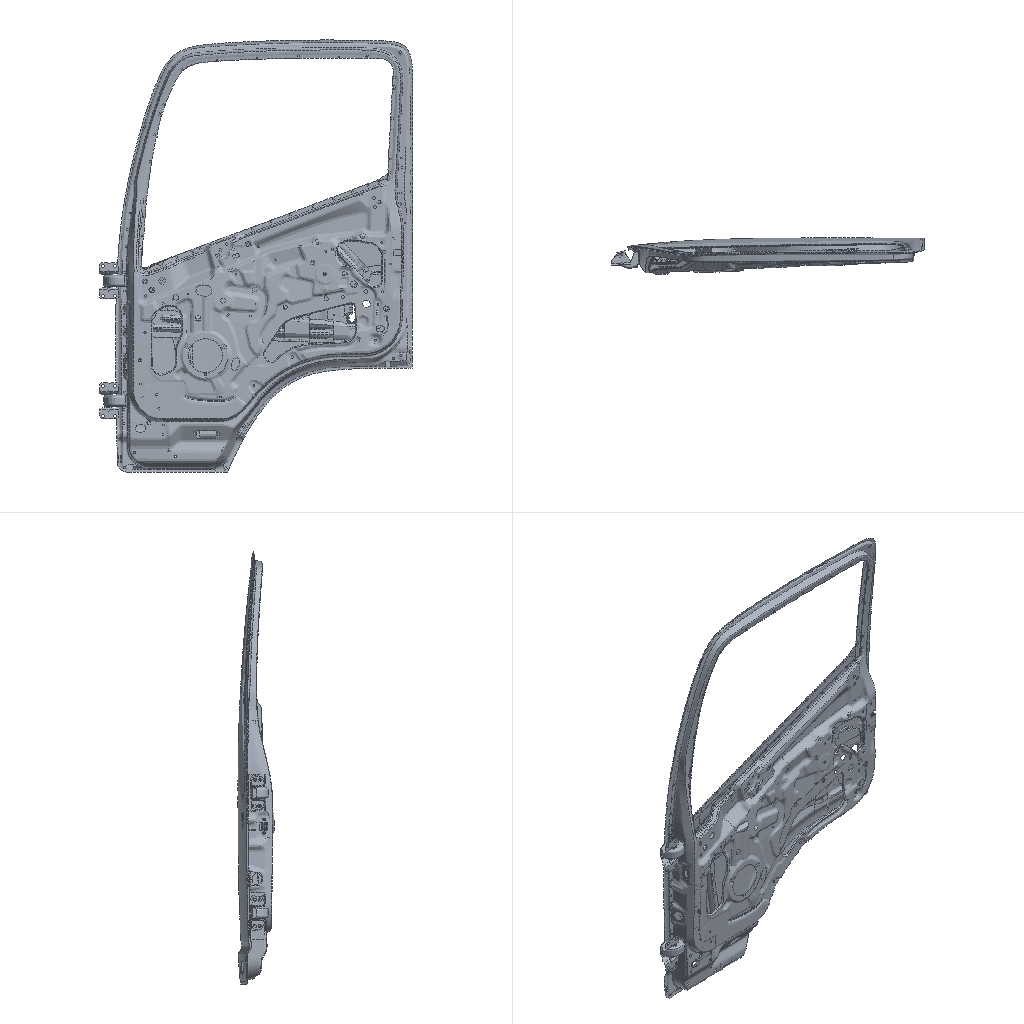Simulation study | nastran
Set-up summary:
category,name,step,type,value,unit,region
solver,nx_nastran
units,not stated in the deck,,not stated
analysis,deck,,static,static
analysis,solution,,SOL,101
load_step,SUBCASE 5,5,SUBCASE,SPC=6 LOAD=7
load_step,SUBCASE 6,6,SUBCASE,SPC=6 LOAD=8
load_step,SUBCASE 7,7,SUBCASE,SPC=6 LOAD=9
load_step,SUBCASE 8,8,SUBCASE,SPC=6 LOAD=10
load_step,SUBCASE 9,9,SUBCASE,SPC=6 LOAD=11
load_step,SUBCASE 10,10,SUBCASE,SPC=6 LOAD=12
load_step,requested,,,6
mesh,nodes,,,45881
mesh,elements,,,43156
element_type,CHEXA,,unverified,162
element_type,CQUAD4,,shell,40635
element_type,CTRIA3,,shell,2521
load,load commands in deck,,count,6
bc,support commands in deck,,count,9
check,setup vs results,,match,"every grid point's frame and coordinates and every element id; grid points of CHEXA, CQUAD4, CTRIA3 elements"
Nastran input file, long lists of numbers shortened:
$$------------------------------------------------------------------------------$
$$                                                                              $
$$ NASTRAN Input Deck Generated by HyperMesh Version  : 9.0b121                 $
$$ Generated using HyperMesh-Nastran Template Version : 9.0b121
$$                                                                              $
$$   Template:  general                                                         $
$$                                                                              $
$$------------------------------------------------------------------------------$
$$------------------------------------------------------------------------------$
$$                      Executive Control Cards                                 $
$$------------------------------------------------------------------------------$
SOL 101
CEND
$$------------------------------------------------------------------------------$
$$                      Case Control Cards                                      $
$$------------------------------------------------------------------------------$
  DISPLACEMENT(PLOT) = ALL
$
$HMNAME LOADSTEP               5"LOADX"
SUBCASE       5
  LABEL=   LOADX
  SPC =        6
  LOAD =        7
$
$HMNAME LOADSTEP               6"LOADY"
SUBCASE       6
  LABEL=   LOADY
  SPC =        6
  LOAD =        8
$
$HMNAME LOADSTEP               7"LOADZ"
SUBCASE       7
  LABEL=   LOADZ
  SPC =        6
  LOAD =        9
$
$HMNAME LOADSTEP               8"LOADX1"
SUBCASE       8
  LABEL= LOADX1
  SPC =        6
  LOAD =       10
$
$HMNAME LOADSTEP               9"LOADY1"
SUBCASE       9
  LABEL= LOADY1
  SPC =        6
  LOAD =       11
$
$HMNAME LOADSTEP              10"LOADZ1"
SUBCASE      10
  LABEL= LOADZ1
  SPC =        6
  LOAD =       12
$$------------------------------------------------------------------------------$
$$                      Bulk Data Cards                                         $
$$------------------------------------------------------------------------------$
BEGIN BULK
PARAM,BAILOUT,-1
PARAM,POST,-1
$$
$$  GRID Data
$$
GRID     1123276        -34.77731037.45 530.3527
GRID     1123277        -35.61231037.5  524.5856
$ (45879 more lines like these left out)
$$
$$  SPOINT Data
$$
$$
$$------------------------------------------------------------------------------$
$$             Group Definitions                                                $
$$------------------------------------------------------------------------------$
$$
$$ RBE2 Elements - Multiple dependent nodes
$$
RBE2     1220176 1190137  123456 1166240 1166241 1166242 1166243 1166244+
+        1166245 1183947 1183948 1183949 1184020
RBE2     1220177 1190138  123456 1166101 1166102 1166103 1166104 1166105+
+        1166106 1183564 1183565 1183566 1183570
$ (91 more lines like these left out)
$
$HMMOVE 61010301
$        1220176THRU     1220179
$
$
$HMMOVE 61010302
$        1220167THRU     1220170 1220172THRU     1220175 1220180THRU     1220182
$        1220184THRU     1220187
$
$
$  RBE3 Elements
$
RBE3     1218917         1188764  1234560.323145     123 11679070.37815 +
+            123 11523500.161067     123 11523490.137638     123 1167906
RBE3     1218918         1188765  1234560.300895     123 11678230.508742+
+            123 11679070.119616     123 11679060.070747     123 1167822
$ (2236 more lines like these left out)
$
$HMMOVE 61010303
$        1218917THRU     1218924 1218926THRU     1218933 1218935THRU     1218942
$        1218944THRU     1218951 1218953THRU     1218960 1218962THRU     1218969
$ (58 more lines like these left out)
CTRIA3   1097712       1 1123279 1123290 1123280
CTRIA3   1097713       1 1123283 1123291 1123284
$ (2519 more lines like these left out)
$
$HMMOVE 61010010
$        1097712THRU     1097713 1097721THRU     1097722 1097725THRU     1097732
$        1097735THRU     1097738 1099905 1100072 1100094 1100145 1100170 1100189
$ (400 more lines like these left out)
CQUAD4   1112534       1 1139953 1140107 1140115 1139952
CQUAD4   1112535       1 1140107 1140108 1140116 1140115
$ (40633 more lines like these left out)
$
$HMMOVE 61010010
$        1112534THRU     1112535 1112541THRU     1112542 1112544 1112546 1112548
$        1112550 1112555THRU     1112557 1112559THRU     1112560 1112562THRU
$ (2064 more lines like these left out)
CHEXA    1218889      12 1188730 1188733 1188732 1188731 1188734 1188737+
+        1188736 1188735
CHEXA    1218898      12 1188740 1188743 1188742 1188741 1188744 1188747+
+        1188746 1188745
$ (320 more lines like these left out)
$
$HMMOVE 61010304
$        1218889 1218898 1218907 1218916 1218925 1218934 1218943 1218952 1218961
$        1218970 1218979 1218988 1218997 1219006 1219015 1219020 1219029 1219038
$ (161 more lines like these left out)
PSHELL         9       14.5            1               1
$
$HMNAME PROP                   8"Pshell400T" 4
$HWCOLOR PROP                  8      13
PSHELL         8       14.0            1               1
$
$HMNAME PROP                   7"Pshell240T" 4
$HWCOLOR PROP                  7       9
PSHELL         7       12.4            1               1
$
$HMNAME PROP                   6"Pshell200T" 4
$HWCOLOR PROP                  6       8
PSHELL         6       12.0            1               1
$
$HMNAME PROP                   5"Pshell150T" 4
$HWCOLOR PROP                  5       7
PSHELL         5       11.5            1               1
$
$HMNAME PROP                   4"Pshell120T" 4
$HWCOLOR PROP                  4       6
PSHELL         4       11.2            1               1
$
$HMNAME PROP                   3"Pshell100T" 4
$HWCOLOR PROP                  3       5
PSHELL         3       11.0            1               1
$
$HMNAME PROP                   2"Pshell70T" 4
$HWCOLOR PROP                  2       4
PSHELL         2       10.7            1               1
$        1219914 1219905 1219896 1219887 1219882 1220061 1219873 1219868 121985
$        1219854 1219845 1219836 1219827 1219822 1219813 1220052 1219808 121979
$        1219790 1219781 1219772 1219763 1219758 1219749 1220043 1219744 121973
$        1219726 1219717 1219708 1219699 1220034 1219690 1219681 1219672 122002
$        1219663 1219654 1219645 1219636 1220024 1219627 1219618 1219609 121960
$        1219591 1219582 1220015 1219573 1219564 1219555 1219546 1220010 121953
$        1219532 1219523 1219518 1219509 1220005 1219504 1219495 1219490 121948
$        1219476 1219467 1219462 1219453 1219448 1219439 1219996 1219434 121942
$        1219420 1219411 1219991 1219402 1219393 1219384 1219375 1219366 121935
$        1219982 1219348 1219339 1219330 1219321 1219312 1219307 1219298 121929
$        1219973 1219284 1219275 1219266 1219257 1219252 1219247 1219238 121923
$        1219228 1219219 1219964 1219210 1219201 1219196 1219187 1219182 121917
$        1219168 1219159 1219154 1219955 1219145 1219140 1219131 1219126 121911
$        1219112 1219103 1219098 1219089 1219946 1219084 1219075 1219070 121906
$        1219056 1219047 1219038 1219029 1219937 1219020 1219015 1219006 121899
$        1218988 1218979 1218970 1218961 1219928 1218952 1218943 1218934 121892
$        1218916 1218907 1219919 1218898 1218889 1220070 1220075 1220080 122008
$        1220094 1220099 1220108 1220117 1220126 1220135 1220144 1220153 122016
$
$
$HMNAME PROP                   1"Pshell80T" 4
$HWCOLOR PROP                  1       3
PSHELL         1       10.8            1               1
$$
$$  PSOLID Data
$
$HMNAME PROP                  12"HEX" 5
$HWCOLOR PROP                 12      20
PSOLID        12       1
$$
$$------------------------------------------------------------------------------$
$$                      Material Definition Cards                               $
$$------------------------------------------------------------------------------$
$$--------------------------------------------------------------
$$ HYPERMESH TAGS
$$--------------------------------------------------------------
$$BEGIN TAGS
$$END TAGS
$$
$$  MAT1 Data
$
$HMNAME MAT                    1"steel" "MAT1"
$HWCOLOR MAT                   1       3
MAT1           1210000.0        0.3     7.90E-09
$$
$$
$$
$$------------------------------------------------------------------------------$
$ (54 more lines like these left out)
SPC            684122187  1234560.0
SPC            6 1190128  1234560.0
SPC            6 1190129  1234560.0
SPC            6 1190130  1234560.0
SPC            6 1190131  1234560.0
SPC            6 1190133  1234560.0
SPC            6 1190134  1234560.0
SPC            6 1190135  1234560.0
SPC            6 1190136  1234560.0
$$
$$  FORCE Data
$$
FORCE          7 1190146       01.0     100.0   0.0     0.0
FORCE          8 1190146       01.0     0.0     100.0   0.0
FORCE          9 1190146       01.0     0.0     0.0     100.0
FORCE         1084122188       01.0     100.0   0.0     0.0
FORCE         1184122188       01.0     0.0     100.0   0.0
FORCE         1284122188       01.0     0.0     0.0     100.0
$HMASSEM 6101010       3 6101010
$HMASSEM_IDS    6101027061010280610100106101010061010020610102006101015061010190
$HMASSEM_IDS    6101012061010050610102906101003061010160610101706101009061010060
$HMASSEM_IDS    6101004061010220610102106101023061010140610100806101013061010070
$HMASSEM_IDS    610102606101018061010250610101106101024061010300
$
ENDDATA
Results summary:
result,analysis,,,static
result,last_loadstep,,,6
result,primary field,,,displacements
result,max displacement,,,1.427,model units